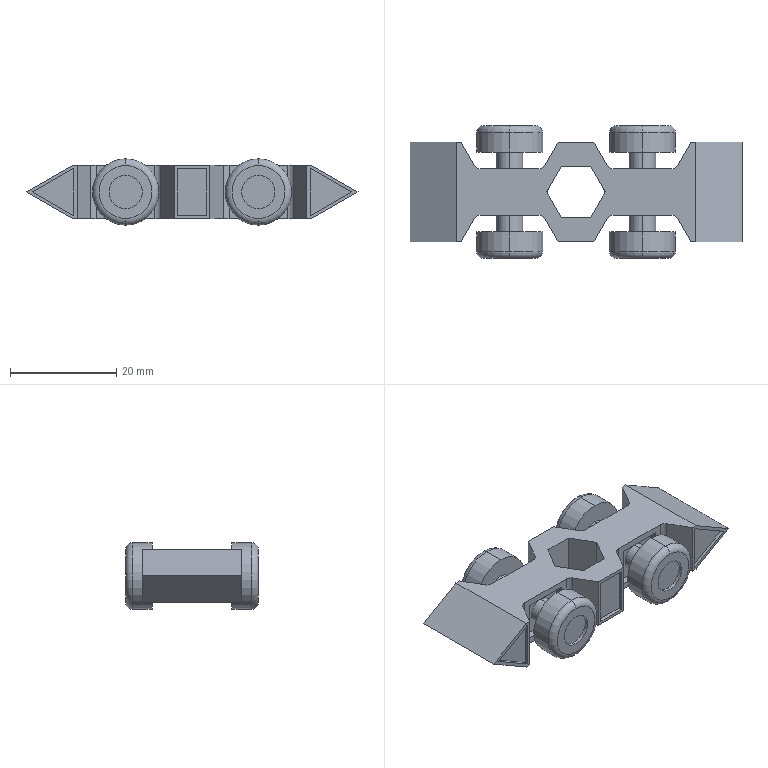Part | SolidWorks | features ICE 8, MirrorPattern 3, Chamfer 1, Extrusion 1, Fillet 1, Scale 1 | 1 solid | 136 faces | box 62.5 x 25 x 12.5 mm | volume 8442 mm3 | plane 96 | cylinder 32 | torus 8 | commonest cylinder face diameters 2.5 x8 5 x8 6.25 x8 12.5 x8